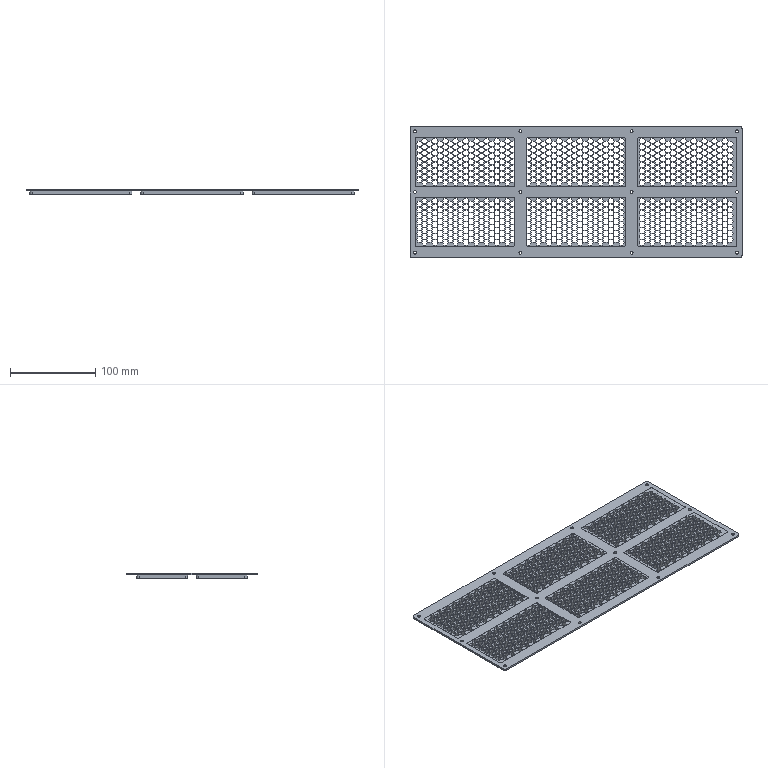NC program | NX | posted with a generic post
Lines 3670 to 4524 of 172913:
(CAVITY_MILL , TOOL : D3_ROUGH)
N7314 T12 M6
N7316 G54
N7318 G17 G0 G90 X-85.591 Y-50.877 S5500 M3
N7320 G43 Z20. H12
N7322 Z1.
N7324 G94 G1 X-85.511 Z0.998 F800.
N7326 X-84.68 Y-49.437 Z0.954
N7328 X-85.511 Y-47.997 Z0.911
N7330 X-87.174 Z0.867
N7332 X-88.006 Y-49.437 Z0.824
N7334 X-87.174 Y-50.877 Z0.78
N7336 X-85.511 Z0.737
N7338 X-84.68 Y-49.437 Z0.693
N7340 X-85.511 Y-47.997 Z0.65
N7342 X-87.174 Z0.606
N7344 X-88.006 Y-49.437 Z0.563
N7346 X-87.174 Y-50.877 Z0.519
N7348 X-85.511 Z0.475
N7350 X-84.68 Y-49.437 Z0.432
N7352 X-85.511 Y-47.997 Z0.388
N7354 X-87.174 Z0.345
N7356 X-88.006 Y-49.437 Z0.301
N7358 X-87.174 Y-50.877 Z0.258
N7360 X-85.511 Z0.214
N7362 X-84.68 Y-49.437 Z0.171
N7364 X-85.511 Y-47.997 Z0.127
N7366 X-87.174 Z0.084
N7368 X-88.006 Y-49.437 Z0.04
N7370 X-87.174 Y-50.877 Z-0.004
N7372 X-85.511 Z-0.047
N7374 X-84.68 Y-49.437 Z-0.091
N7376 X-85.511 Y-47.997 Z-0.134
N7378 X-87.174 Z-0.178
N7380 X-88.006 Y-49.437 Z-0.221
N7382 X-87.174 Y-50.877 Z-0.265
N7384 X-85.511 Z-0.308
N7386 X-84.68 Y-49.437 Z-0.352
N7388 X-85.511 Y-47.997 Z-0.395
N7390 X-87.174 Z-0.439
N7392 X-88.006 Y-49.437 Z-0.482
N7394 X-87.174 Y-50.877 Z-0.526
N7396 X-85.511 Z-0.57
N7398 X-84.68 Y-49.437 Z-0.613
N7400 X-85.511 Y-47.997 Z-0.657
N7402 X-87.174 Z-0.7
N7404 X-88.006 Y-49.437 Z-0.744
N7406 X-87.174 Y-50.877 Z-0.787
N7408 X-85.511 Z-0.831
N7410 X-84.68 Y-49.437 Z-0.874
N7412 X-85.511 Y-47.997 Z-0.918
N7414 X-87.174 Z-0.961
N7416 X-88.006 Y-49.437 Z-1.005
N7418 X-87.174 Y-50.877 Z-1.049
N7420 X-85.511 Z-1.092
N7422 X-84.68 Y-49.437 Z-1.136
N7424 X-85.511 Y-47.997 Z-1.179
N7426 X-87.174 Z-1.223
N7428 X-88.006 Y-49.437 Z-1.266
N7430 X-87.174 Y-50.877 Z-1.31
N7432 X-85.511 Z-1.353
N7434 X-84.68 Y-49.437 Z-1.397
N7436 X-85.511 Y-47.997 Z-1.44
N7438 X-87.174 Z-1.484
N7440 X-88.006 Y-49.437 Z-1.527
N7442 X-87.174 Y-50.877 Z-1.571
N7444 X-85.511 Z-1.615
N7446 X-84.68 Y-49.437 Z-1.658
N7448 X-85.511 Y-47.997 Z-1.702
N7450 X-87.174 Z-1.745
N7452 X-88.006 Y-49.437 Z-1.789
N7454 X-87.174 Y-50.877 Z-1.832
N7456 X-85.511 Z-1.876
N7458 X-84.68 Y-49.437 Z-1.919
N7460 X-85.511 Y-47.997 Z-1.963
N7462 X-87.174 Z-2.006
N7464 X-88.006 Y-49.437 Z-2.05
N7466 X-87.174 Y-50.877 Z-2.093
N7468 X-85.511 Z-2.137
N7470 X-84.68 Y-49.437 Z-2.181
N7472 X-85.511 Y-47.997 Z-2.224
N7474 X-87.174 Z-2.268
N7476 X-88.006 Y-49.437 Z-2.311
N7478 X-87.174 Y-50.877 Z-2.355
N7480 X-85.511 Z-2.398
N7482 X-84.68 Y-49.437 Z-2.442
N7484 X-85.511 Y-47.997 Z-2.485
N7486 X-87.174 Z-2.529
N7488 X-88.006 Y-49.437 Z-2.572
N7490 X-87.174 Y-50.877 Z-2.616
N7492 X-85.511 Z-2.66
N7494 X-84.68 Y-49.437 Z-2.703
N7496 X-85.511 Y-47.997 Z-2.747
N7498 X-87.174 Z-2.79
N7500 X-88.006 Y-49.437 Z-2.834
N7502 X-87.174 Y-50.877 Z-2.877
N7504 X-85.511 Z-2.921
N7506 X-84.68 Y-49.437 Z-2.964
N7508 X-85.511 Y-47.997 Z-3.008
N7510 X-87.174 Z-3.051
N7512 X-88.006 Y-49.437 Z-3.095
N7514 X-87.174 Y-50.877 Z-3.138
N7516 X-85.511 Z-3.182
N7518 X-84.68 Y-49.437 Z-3.226
N7520 X-85.511 Y-47.997 Z-3.269
N7522 X-87.174 Z-3.313
N7524 X-88.006 Y-49.437 Z-3.356
N7526 X-87.174 Y-50.877 Z-3.4
N7528 X-85.511 Z-3.443
N7530 X-84.68 Y-49.437 Z-3.487
N7532 X-85.511 Y-47.997 Z-3.53
N7534 X-87.174 Z-3.574
N7536 X-88.006 Y-49.437 Z-3.617
N7538 X-87.174 Y-50.877 Z-3.661
N7540 X-85.511 Z-3.705
N7542 X-84.68 Y-49.437 Z-3.748
N7544 X-85.511 Y-47.997 Z-3.792
N7546 X-87.174 Z-3.835
N7548 X-88.006 Y-49.437 Z-3.879
N7550 X-87.174 Y-50.877 Z-3.922
N7552 X-85.511 Z-3.966
N7554 X-84.68 Y-49.437 Z-4.009
N7556 X-85.511 Y-47.997 Z-4.053
N7558 X-87.174 Z-4.096
N7560 X-88.006 Y-49.437 Z-4.14
N7562 X-87.174 Y-50.877 Z-4.183
N7564 X-85.511 Z-4.227
N7566 X-84.68 Y-49.437 Z-4.271
N7568 X-85.511 Y-47.997 Z-4.314
N7570 X-87.174 Z-4.358
N7572 X-88.006 Y-49.437 Z-4.401
N7574 X-87.174 Y-50.877 Z-4.445
N7576 X-85.511 Z-4.488
N7578 X-84.68 Y-49.437 Z-4.532
N7580 X-85.511 Y-47.997 Z-4.575
N7582 X-87.174 Z-4.619
N7584 X-88.006 Y-49.437 Z-4.662
N7586 X-87.174 Y-50.877 Z-4.706
N7588 X-85.511 Z-4.75
N7590 X-84.68 Y-49.437 Z-4.793
N7592 X-85.511 Y-47.997 Z-4.837
N7594 X-87.174 Z-4.88
N7596 X-88.006 Y-49.437 Z-4.924
N7598 X-87.174 Y-50.877 Z-4.967
N7600 X-85.511 Z-5.011
N7602 X-84.68 Y-49.437 Z-5.054
N7604 X-85.511 Y-47.997 Z-5.098
N7606 X-87.174 Z-5.141
N7608 X-88.006 Y-49.437 Z-5.185
N7610 X-87.174 Y-50.877 Z-5.228
N7612 X-85.511 Z-5.272
N7614 X-84.68 Y-49.437 Z-5.316
N7616 X-85.511 Y-47.997 Z-5.359
N7618 X-87.174 Z-5.403
N7620 X-88.006 Y-49.437 Z-5.446
N7622 X-87.174 Y-50.877 Z-5.49
N7624 X-85.511 Z-5.533
N7626 X-84.68 Y-49.437 Z-5.577
N7628 X-85.511 Y-47.997 Z-5.62
N7630 X-87.174 Z-5.664
N7632 X-88.006 Y-49.437 Z-5.707
N7634 X-87.174 Y-50.877 Z-5.751
N7636 X-85.511 Z-5.794
N7638 X-84.68 Y-49.437 Z-5.838
N7640 X-85.511 Y-47.997 Z-5.882
N7642 X-87.174 Z-5.925
N7644 X-88.006 Y-49.437 Z-5.969
N7646 X-87.174 Y-50.877 Z-6.012
N7648 X-85.511 Z-6.056
N7650 X-84.68 Y-49.437 Z-6.099
N7652 X-85.511 Y-47.997 Z-6.143
N7654 X-87.174 Z-6.186
N7656 X-88.006 Y-49.437 Z-6.23
N7658 X-87.174 Y-50.877 Z-6.273
N7660 X-85.511 Z-6.317
N7662 X-84.68 Y-49.437 Z-6.361
N7664 X-85.511 Y-47.997 Z-6.404
N7666 X-87.174 Z-6.448
N7668 X-88.006 Y-49.437 Z-6.491
N7670 X-87.174 Y-50.877 Z-6.535
N7672 X-85.511 Z-6.578
N7674 X-85.096 Y-50.157 Z-6.6
N7676 X-84.68 Y-49.437
N7678 X-85.511 Y-47.997
N7680 X-87.174
N7682 X-88.006 Y-49.437
N7684 X-87.174 Y-50.877
N7686 X-85.511
N7688 X-85.096 Y-50.157
N7690 Z-5.6
N7692 G0 Z20.
N7694 X-87.214 Y-43.809
N7696 Z1.
N7698 G1 X-87.174 Y-43.877 Z0.998
N7700 X-85.511 Z0.954
N7702 X-84.68 Y-42.437 Z0.911
N7704 X-85.511 Y-40.997 Z0.867
N7706 X-87.174 Z0.824
N7708 X-88.006 Y-42.437 Z0.78
N7710 X-87.174 Y-43.877 Z0.737
N7712 X-85.511 Z0.693
N7714 X-84.68 Y-42.437 Z0.65
N7716 X-85.511 Y-40.997 Z0.606
N7718 X-87.174 Z0.563
N7720 X-88.006 Y-42.437 Z0.519
N7722 X-87.174 Y-43.877 Z0.475
N7724 X-85.511 Z0.432
N7726 X-84.68 Y-42.437 Z0.388
N7728 X-85.511 Y-40.997 Z0.345
N7730 X-87.174 Z0.301
N7732 X-88.006 Y-42.437 Z0.258
N7734 X-87.174 Y-43.877 Z0.214
N7736 X-85.511 Z0.171
N7738 X-84.68 Y-42.437 Z0.127
N7740 X-85.511 Y-40.997 Z0.084
N7742 X-87.174 Z0.04
N7744 X-88.006 Y-42.437 Z-0.004
N7746 X-87.174 Y-43.877 Z-0.047
N7748 X-85.511 Z-0.091
N7750 X-84.68 Y-42.437 Z-0.134
N7752 X-85.511 Y-40.997 Z-0.178
N7754 X-87.174 Z-0.221
N7756 X-88.006 Y-42.437 Z-0.265
N7758 X-87.174 Y-43.877 Z-0.308
N7760 X-85.511 Z-0.352
N7762 X-84.68 Y-42.437 Z-0.395
N7764 X-85.511 Y-40.997 Z-0.439
N7766 X-87.174 Z-0.482
N7768 X-88.006 Y-42.437 Z-0.526
N7770 X-87.174 Y-43.877 Z-0.57
N7772 X-85.511 Z-0.613
N7774 X-84.68 Y-42.437 Z-0.657
N7776 X-85.511 Y-40.997 Z-0.7
N7778 X-87.174 Z-0.744
N7780 X-88.006 Y-42.437 Z-0.787
N7782 X-87.174 Y-43.877 Z-0.831
N7784 X-85.511 Z-0.874
N7786 X-84.68 Y-42.437 Z-0.918
N7788 X-85.511 Y-40.997 Z-0.961
N7790 X-87.174 Z-1.005
N7792 X-88.006 Y-42.437 Z-1.049
N7794 X-87.174 Y-43.877 Z-1.092
N7796 X-85.511 Z-1.136
N7798 X-84.68 Y-42.437 Z-1.179
N7800 X-85.511 Y-40.997 Z-1.223
N7802 X-87.174 Z-1.266
N7804 X-88.006 Y-42.437 Z-1.31
N7806 X-87.174 Y-43.877 Z-1.353
N7808 X-85.511 Z-1.397
N7810 X-84.68 Y-42.437 Z-1.44
N7812 X-85.511 Y-40.997 Z-1.484
N7814 X-87.174 Z-1.527
N7816 X-88.006 Y-42.437 Z-1.571
N7818 X-87.174 Y-43.877 Z-1.615
N7820 X-85.511 Z-1.658
N7822 X-84.68 Y-42.437 Z-1.702
N7824 X-85.511 Y-40.997 Z-1.745
N7826 X-87.174 Z-1.789
N7828 X-88.006 Y-42.437 Z-1.832
N7830 X-87.174 Y-43.877 Z-1.876
N7832 X-85.511 Z-1.919
N7834 X-84.68 Y-42.437 Z-1.963
N7836 X-85.511 Y-40.997 Z-2.006
N7838 X-87.174 Z-2.05
N7840 X-88.006 Y-42.437 Z-2.093
N7842 X-87.174 Y-43.877 Z-2.137
N7844 X-85.511 Z-2.181
N7846 X-84.68 Y-42.437 Z-2.224
N7848 X-85.511 Y-40.997 Z-2.268
N7850 X-87.174 Z-2.311
N7852 X-88.006 Y-42.437 Z-2.355
N7854 X-87.174 Y-43.877 Z-2.398
N7856 X-85.511 Z-2.442
N7858 X-84.68 Y-42.437 Z-2.485
N7860 X-85.511 Y-40.997 Z-2.529
N7862 X-87.174 Z-2.572
N7864 X-88.006 Y-42.437 Z-2.616
N7866 X-87.174 Y-43.877 Z-2.66
N7868 X-85.511 Z-2.703
N7870 X-84.68 Y-42.437 Z-2.747
N7872 X-85.511 Y-40.997 Z-2.79
N7874 X-87.174 Z-2.834
N7876 X-88.006 Y-42.437 Z-2.877
N7878 X-87.174 Y-43.877 Z-2.921
N7880 X-85.511 Z-2.964
N7882 X-84.68 Y-42.437 Z-3.008
N7884 X-85.511 Y-40.997 Z-3.051
N7886 X-87.174 Z-3.095
N7888 X-88.006 Y-42.437 Z-3.138
N7890 X-87.174 Y-43.877 Z-3.182
N7892 X-85.511 Z-3.226
N7894 X-84.68 Y-42.437 Z-3.269
N7896 X-85.511 Y-40.997 Z-3.313
N7898 X-87.174 Z-3.356
N7900 X-88.006 Y-42.437 Z-3.4
N7902 X-87.174 Y-43.877 Z-3.443
N7904 X-85.511 Z-3.487
N7906 X-84.68 Y-42.437 Z-3.53
N7908 X-85.511 Y-40.997 Z-3.574
N7910 X-87.174 Z-3.617
N7912 X-88.006 Y-42.437 Z-3.661
N7914 X-87.174 Y-43.877 Z-3.705
N7916 X-85.511 Z-3.748
N7918 X-84.68 Y-42.437 Z-3.792
N7920 X-85.511 Y-40.997 Z-3.835
N7922 X-87.174 Z-3.879
N7924 X-88.006 Y-42.437 Z-3.922
N7926 X-87.174 Y-43.877 Z-3.966
N7928 X-85.511 Z-4.009
N7930 X-84.68 Y-42.437 Z-4.053
N7932 X-85.511 Y-40.997 Z-4.096
N7934 X-87.174 Z-4.14
N7936 X-88.006 Y-42.437 Z-4.183
N7938 X-87.174 Y-43.877 Z-4.227
N7940 X-85.511 Z-4.271
N7942 X-84.68 Y-42.437 Z-4.314
N7944 X-85.511 Y-40.997 Z-4.358
N7946 X-87.174 Z-4.401
N7948 X-88.006 Y-42.437 Z-4.445
N7950 X-87.174 Y-43.877 Z-4.488
N7952 X-85.511 Z-4.532
N7954 X-84.68 Y-42.437 Z-4.575
N7956 X-85.511 Y-40.997 Z-4.619
N7958 X-87.174 Z-4.662
N7960 X-88.006 Y-42.437 Z-4.706
N7962 X-87.174 Y-43.877 Z-4.75
N7964 X-85.511 Z-4.793
N7966 X-84.68 Y-42.437 Z-4.837
N7968 X-85.511 Y-40.997 Z-4.88
N7970 X-87.174 Z-4.924
N7972 X-88.006 Y-42.437 Z-4.967
N7974 X-87.174 Y-43.877 Z-5.011
N7976 X-85.511 Z-5.054
N7978 X-84.68 Y-42.437 Z-5.098
N7980 X-85.511 Y-40.997 Z-5.141
N7982 X-87.174 Z-5.185
N7984 X-88.006 Y-42.437 Z-5.228
N7986 X-87.174 Y-43.877 Z-5.272
N7988 X-85.511 Z-5.316
N7990 X-84.68 Y-42.437 Z-5.359
N7992 X-85.511 Y-40.997 Z-5.403
N7994 X-87.174 Z-5.446
N7996 X-88.006 Y-42.437 Z-5.49
N7998 X-87.174 Y-43.877 Z-5.533
N8000 X-85.511 Z-5.577
N8002 X-84.68 Y-42.437 Z-5.62
N8004 X-85.511 Y-40.997 Z-5.664
N8006 X-87.174 Z-5.707
N8008 X-88.006 Y-42.437 Z-5.751
N8010 X-87.174 Y-43.877 Z-5.794
N8012 X-85.511 Z-5.838
N8014 X-84.68 Y-42.437 Z-5.882
N8016 X-85.511 Y-40.997 Z-5.925
N8018 X-87.174 Z-5.969
N8020 X-88.006 Y-42.437 Z-6.012
N8022 X-87.174 Y-43.877 Z-6.056
N8024 X-85.511 Z-6.099
N8026 X-84.68 Y-42.437 Z-6.143
N8028 X-85.511 Y-40.997 Z-6.186
N8030 X-87.174 Z-6.23
N8032 X-88.006 Y-42.437 Z-6.273
N8034 X-87.174 Y-43.877 Z-6.317
N8036 X-85.511 Z-6.361
N8038 X-84.68 Y-42.437 Z-6.404
N8040 X-85.511 Y-40.997 Z-6.448
N8042 X-87.174 Z-6.491
N8044 X-88.006 Y-42.437 Z-6.535
N8046 X-87.174 Y-43.877 Z-6.578
N8048 X-86.343 Z-6.6
N8050 X-85.511
N8052 X-84.68 Y-42.437
N8054 X-85.511 Y-40.997
N8056 X-87.174
N8058 X-88.006 Y-42.437
N8060 X-87.174 Y-43.877
N8062 X-86.343
N8064 Z-5.6
N8066 G0 Z20.
N8068 X-91.653 Y-47.377
N8070 Z1.
N8072 G1 X-91.574 Z0.998
N8074 X-90.742 Y-45.937 Z0.954
N8076 X-91.574 Y-44.497 Z0.911
N8078 X-93.236 Z0.867
N8080 X-94.068 Y-45.937 Z0.824
N8082 X-93.236 Y-47.377 Z0.78
N8084 X-91.574 Z0.737
N8086 X-90.742 Y-45.937 Z0.693
N8088 X-91.574 Y-44.497 Z0.65
N8090 X-93.236 Z0.606
N8092 X-94.068 Y-45.937 Z0.563
N8094 X-93.236 Y-47.377 Z0.519
N8096 X-91.574 Z0.475
N8098 X-90.742 Y-45.937 Z0.432
N8100 X-91.574 Y-44.497 Z0.388
N8102 X-93.236 Z0.345
N8104 X-94.068 Y-45.937 Z0.301
N8106 X-93.236 Y-47.377 Z0.258
N8108 X-91.574 Z0.214
N8110 X-90.742 Y-45.937 Z0.171
N8112 X-91.574 Y-44.497 Z0.127
N8114 X-93.236 Z0.084
N8116 X-94.068 Y-45.937 Z0.04
N8118 X-93.236 Y-47.377 Z-0.004
N8120 X-91.574 Z-0.047
N8122 X-90.742 Y-45.937 Z-0.091
N8124 X-91.574 Y-44.497 Z-0.134
N8126 X-93.236 Z-0.178
N8128 X-94.068 Y-45.937 Z-0.221
N8130 X-93.236 Y-47.377 Z-0.265
N8132 X-91.574 Z-0.308
N8134 X-90.742 Y-45.937 Z-0.352
N8136 X-91.574 Y-44.497 Z-0.395
N8138 X-93.236 Z-0.439
N8140 X-94.068 Y-45.937 Z-0.482
N8142 X-93.236 Y-47.377 Z-0.526
N8144 X-91.574 Z-0.57
N8146 X-90.742 Y-45.937 Z-0.613
N8148 X-91.574 Y-44.497 Z-0.657
N8150 X-93.236 Z-0.7
N8152 X-94.068 Y-45.937 Z-0.744
N8154 X-93.236 Y-47.377 Z-0.787
N8156 X-91.574 Z-0.831
N8158 X-90.742 Y-45.937 Z-0.874
N8160 X-91.574 Y-44.497 Z-0.918
N8162 X-93.236 Z-0.961
N8164 X-94.068 Y-45.937 Z-1.005
N8166 X-93.236 Y-47.377 Z-1.049
N8168 X-91.574 Z-1.092
N8170 X-90.742 Y-45.937 Z-1.136
N8172 X-91.574 Y-44.497 Z-1.179
N8174 X-93.236 Z-1.223
N8176 X-94.068 Y-45.937 Z-1.266
N8178 X-93.236 Y-47.377 Z-1.31
N8180 X-91.574 Z-1.353
N8182 X-90.742 Y-45.937 Z-1.397
N8184 X-91.574 Y-44.497 Z-1.44
N8186 X-93.236 Z-1.484
N8188 X-94.068 Y-45.937 Z-1.527
N8190 X-93.236 Y-47.377 Z-1.571
N8192 X-91.574 Z-1.615
N8194 X-90.742 Y-45.937 Z-1.658
N8196 X-91.574 Y-44.497 Z-1.702
N8198 X-93.236 Z-1.745
N8200 X-94.068 Y-45.937 Z-1.789
N8202 X-93.236 Y-47.377 Z-1.832
N8204 X-91.574 Z-1.876
N8206 X-90.742 Y-45.937 Z-1.919
N8208 X-91.574 Y-44.497 Z-1.963
N8210 X-93.236 Z-2.006
N8212 X-94.068 Y-45.937 Z-2.05
N8214 X-93.236 Y-47.377 Z-2.093
N8216 X-91.574 Z-2.137
N8218 X-90.742 Y-45.937 Z-2.181
N8220 X-91.574 Y-44.497 Z-2.224
N8222 X-93.236 Z-2.268
N8224 X-94.068 Y-45.937 Z-2.311
N8226 X-93.236 Y-47.377 Z-2.355
N8228 X-91.574 Z-2.398
N8230 X-90.742 Y-45.937 Z-2.442
N8232 X-91.574 Y-44.497 Z-2.485
N8234 X-93.236 Z-2.529
N8236 X-94.068 Y-45.937 Z-2.572
N8238 X-93.236 Y-47.377 Z-2.616
N8240 X-91.574 Z-2.66
N8242 X-90.742 Y-45.937 Z-2.703
N8244 X-91.574 Y-44.497 Z-2.747
N8246 X-93.236 Z-2.79
N8248 X-94.068 Y-45.937 Z-2.834
N8250 X-93.236 Y-47.377 Z-2.877
N8252 X-91.574 Z-2.921
N8254 X-90.742 Y-45.937 Z-2.964
N8256 X-91.574 Y-44.497 Z-3.008
N8258 X-93.236 Z-3.051
N8260 X-94.068 Y-45.937 Z-3.095
N8262 X-93.236 Y-47.377 Z-3.138
N8264 X-91.574 Z-3.182
N8266 X-90.742 Y-45.937 Z-3.226
N8268 X-91.574 Y-44.497 Z-3.269
N8270 X-93.236 Z-3.313
N8272 X-94.068 Y-45.937 Z-3.356
N8274 X-93.236 Y-47.377 Z-3.4
N8276 X-91.574 Z-3.443
N8278 X-90.742 Y-45.937 Z-3.487
N8280 X-91.574 Y-44.497 Z-3.53
N8282 X-93.236 Z-3.574
N8284 X-94.068 Y-45.937 Z-3.617
N8286 X-93.236 Y-47.377 Z-3.661
N8288 X-91.574 Z-3.705
N8290 X-90.742 Y-45.937 Z-3.748
N8292 X-91.574 Y-44.497 Z-3.792
N8294 X-93.236 Z-3.835
N8296 X-94.068 Y-45.937 Z-3.879
N8298 X-93.236 Y-47.377 Z-3.922
N8300 X-91.574 Z-3.966
N8302 X-90.742 Y-45.937 Z-4.009
N8304 X-91.574 Y-44.497 Z-4.053
N8306 X-93.236 Z-4.096
N8308 X-94.068 Y-45.937 Z-4.14
N8310 X-93.236 Y-47.377 Z-4.183
N8312 X-91.574 Z-4.227
N8314 X-90.742 Y-45.937 Z-4.271
N8316 X-91.574 Y-44.497 Z-4.314
N8318 X-93.236 Z-4.358
N8320 X-94.068 Y-45.937 Z-4.401
N8322 X-93.236 Y-47.377 Z-4.445
N8324 X-91.574 Z-4.488
N8326 X-90.742 Y-45.937 Z-4.532
N8328 X-91.574 Y-44.497 Z-4.575
N8330 X-93.236 Z-4.619
N8332 X-94.068 Y-45.937 Z-4.662
N8334 X-93.236 Y-47.377 Z-4.706
N8336 X-91.574 Z-4.75
N8338 X-90.742 Y-45.937 Z-4.793
N8340 X-91.574 Y-44.497 Z-4.837
N8342 X-93.236 Z-4.88
N8344 X-94.068 Y-45.937 Z-4.924
N8346 X-93.236 Y-47.377 Z-4.967
N8348 X-91.574 Z-5.011
N8350 X-90.742 Y-45.937 Z-5.054
N8352 X-91.574 Y-44.497 Z-5.098
N8354 X-93.236 Z-5.141
N8356 X-94.068 Y-45.937 Z-5.185
N8358 X-93.236 Y-47.377 Z-5.228
N8360 X-91.574 Z-5.272
N8362 X-90.742 Y-45.937 Z-5.316
N8364 X-91.574 Y-44.497 Z-5.359
N8366 X-93.236 Z-5.403
N8368 X-94.068 Y-45.937 Z-5.446
N8370 X-93.236 Y-47.377 Z-5.49
N8372 X-91.574 Z-5.533
N8374 X-90.742 Y-45.937 Z-5.577
N8376 X-91.574 Y-44.497 Z-5.62
N8378 X-93.236 Z-5.664
N8380 X-94.068 Y-45.937 Z-5.707
N8382 X-93.236 Y-47.377 Z-5.751
N8384 X-91.574 Z-5.794
N8386 X-90.742 Y-45.937 Z-5.838
N8388 X-91.574 Y-44.497 Z-5.882
N8390 X-93.236 Z-5.925
N8392 X-94.068 Y-45.937 Z-5.969
N8394 X-93.236 Y-47.377 Z-6.012
N8396 X-91.574 Z-6.056
N8398 X-90.742 Y-45.937 Z-6.099
N8400 X-91.574 Y-44.497 Z-6.143
N8402 X-93.236 Z-6.186
N8404 X-94.068 Y-45.937 Z-6.23
N8406 X-93.236 Y-47.377 Z-6.273
N8408 X-91.574 Z-6.317
N8410 X-90.742 Y-45.937 Z-6.361
N8412 X-91.574 Y-44.497 Z-6.404
N8414 X-93.236 Z-6.448
N8416 X-94.068 Y-45.937 Z-6.491
N8418 X-93.236 Y-47.377 Z-6.535
N8420 X-91.574 Z-6.578
N8422 X-91.158 Y-46.657 Z-6.6
N8424 X-90.742 Y-45.937
N8426 X-91.574 Y-44.497
N8428 X-93.236
N8430 X-94.068 Y-45.937
N8432 X-93.236 Y-47.377
N8434 X-91.574
N8436 X-91.158 Y-46.657
N8438 Z-5.6
N8440 G0 Z20.
N8442 X-93.276 Y-54.309
N8444 Z1.
N8446 G1 X-93.236 Y-54.377 Z0.998
N8448 X-91.574 Z0.954
N8450 X-90.742 Y-52.937 Z0.911
N8452 X-91.574 Y-51.497 Z0.867
N8454 X-93.236 Z0.824
N8456 X-94.068 Y-52.937 Z0.78
N8458 X-93.236 Y-54.377 Z0.737
N8460 X-91.574 Z0.693
N8462 X-90.742 Y-52.937 Z0.65
N8464 X-91.574 Y-51.497 Z0.606
N8466 X-93.236 Z0.563
N8468 X-94.068 Y-52.937 Z0.519
N8470 X-93.236 Y-54.377 Z0.475
N8472 X-91.574 Z0.432
N8474 X-90.742 Y-52.937 Z0.388
N8476 X-91.574 Y-51.497 Z0.345
N8478 X-93.236 Z0.301
N8480 X-94.068 Y-52.937 Z0.258
N8482 X-93.236 Y-54.377 Z0.214
N8484 X-91.574 Z0.171
N8486 X-90.742 Y-52.937 Z0.127
N8488 X-91.574 Y-51.497 Z0.084
N8490 X-93.236 Z0.04
N8492 X-94.068 Y-52.937 Z-0.004
N8494 X-93.236 Y-54.377 Z-0.047
N8496 X-91.574 Z-0.091
N8498 X-90.742 Y-52.937 Z-0.134
N8500 X-91.574 Y-51.497 Z-0.178
N8502 X-93.236 Z-0.221
N8504 X-94.068 Y-52.937 Z-0.265
N8506 X-93.236 Y-54.377 Z-0.308
N8508 X-91.574 Z-0.352
N8510 X-90.742 Y-52.937 Z-0.395
N8512 X-91.574 Y-51.497 Z-0.439
N8514 X-93.236 Z-0.482
N8516 X-94.068 Y-52.937 Z-0.526
N8518 X-93.236 Y-54.377 Z-0.57
N8520 X-91.574 Z-0.613
N8522 X-90.742 Y-52.937 Z-0.657
N8524 X-91.574 Y-51.497 Z-0.7
N8526 X-93.236 Z-0.744
N8528 X-94.068 Y-52.937 Z-0.787
N8530 X-93.236 Y-54.377 Z-0.831
N8532 X-91.574 Z-0.874
N8534 X-90.742 Y-52.937 Z-0.918
N8536 X-91.574 Y-51.497 Z-0.961
N8538 X-93.236 Z-1.005
N8540 X-94.068 Y-52.937 Z-1.049
N8542 X-93.236 Y-54.377 Z-1.092
N8544 X-91.574 Z-1.136
N8546 X-90.742 Y-52.937 Z-1.179
N8548 X-91.574 Y-51.497 Z-1.223
N8550 X-93.236 Z-1.266
N8552 X-94.068 Y-52.937 Z-1.31
N8554 X-93.236 Y-54.377 Z-1.353
N8556 X-91.574 Z-1.397
N8558 X-90.742 Y-52.937 Z-1.44
N8560 X-91.574 Y-51.497 Z-1.484
N8562 X-93.236 Z-1.527
N8564 X-94.068 Y-52.937 Z-1.571
N8566 X-93.236 Y-54.377 Z-1.615
N8568 X-91.574 Z-1.658
N8570 X-90.742 Y-52.937 Z-1.702
N8572 X-91.574 Y-51.497 Z-1.745
N8574 X-93.236 Z-1.789
N8576 X-94.068 Y-52.937 Z-1.832
N8578 X-93.236 Y-54.377 Z-1.876
N8580 X-91.574 Z-1.919
N8582 X-90.742 Y-52.937 Z-1.963
N8584 X-91.574 Y-51.497 Z-2.006
N8586 X-93.236 Z-2.05
N8588 X-94.068 Y-52.937 Z-2.093
N8590 X-93.236 Y-54.377 Z-2.137
N8592 X-91.574 Z-2.181
N8594 X-90.742 Y-52.937 Z-2.224
N8596 X-91.574 Y-51.497 Z-2.268
N8598 X-93.236 Z-2.311
N8600 X-94.068 Y-52.937 Z-2.355
N8602 X-93.236 Y-54.377 Z-2.398
N8604 X-91.574 Z-2.442
N8606 X-90.742 Y-52.937 Z-2.485
N8608 X-91.574 Y-51.497 Z-2.529
N8610 X-93.236 Z-2.572
N8612 X-94.068 Y-52.937 Z-2.616
N8614 X-93.236 Y-54.377 Z-2.66
N8616 X-91.574 Z-2.703
N8618 X-90.742 Y-52.937 Z-2.747
N8620 X-91.574 Y-51.497 Z-2.79
N8622 X-93.236 Z-2.834
N8624 X-94.068 Y-52.937 Z-2.877
N8626 X-93.236 Y-54.377 Z-2.921
N8628 X-91.574 Z-2.964
N8630 X-90.742 Y-52.937 Z-3.008
N8632 X-91.574 Y-51.497 Z-3.051
N8634 X-93.236 Z-3.095
N8636 X-94.068 Y-52.937 Z-3.138
N8638 X-93.236 Y-54.377 Z-3.182
N8640 X-91.574 Z-3.226
N8642 X-90.742 Y-52.937 Z-3.269
N8644 X-91.574 Y-51.497 Z-3.313
N8646 X-93.236 Z-3.356
N8648 X-94.068 Y-52.937 Z-3.4
N8650 X-93.236 Y-54.377 Z-3.443
N8652 X-91.574 Z-3.487
N8654 X-90.742 Y-52.937 Z-3.53
N8656 X-91.574 Y-51.497 Z-3.574
N8658 X-93.236 Z-3.617
N8660 X-94.068 Y-52.937 Z-3.661
N8662 X-93.236 Y-54.377 Z-3.705
N8664 X-91.574 Z-3.748
N8666 X-90.742 Y-52.937 Z-3.792
N8668 X-91.574 Y-51.497 Z-3.835
N8670 X-93.236 Z-3.879
N8672 X-94.068 Y-52.937 Z-3.922
N8674 X-93.236 Y-54.377 Z-3.966
N8676 X-91.574 Z-4.009
N8678 X-90.742 Y-52.937 Z-4.053
N8680 X-91.574 Y-51.497 Z-4.096
N8682 X-93.236 Z-4.14
N8684 X-94.068 Y-52.937 Z-4.183
N8686 X-93.236 Y-54.377 Z-4.227
N8688 X-91.574 Z-4.271
N8690 X-90.742 Y-52.937 Z-4.314
N8692 X-91.574 Y-51.497 Z-4.358
N8694 X-93.236 Z-4.401
N8696 X-94.068 Y-52.937 Z-4.445
N8698 X-93.236 Y-54.377 Z-4.488
N8700 X-91.574 Z-4.532
N8702 X-90.742 Y-52.937 Z-4.575
N8704 X-91.574 Y-51.497 Z-4.619
N8706 X-93.236 Z-4.662
N8708 X-94.068 Y-52.937 Z-4.706
N8710 X-93.236 Y-54.377 Z-4.75
N8712 X-91.574 Z-4.793
N8714 X-90.742 Y-52.937 Z-4.837
N8716 X-91.574 Y-51.497 Z-4.88
N8718 X-93.236 Z-4.924
N8720 X-94.068 Y-52.937 Z-4.967
N8722 X-93.236 Y-54.377 Z-5.011
N8724 X-91.574 Z-5.054
N8726 X-90.742 Y-52.937 Z-5.098
N8728 X-91.574 Y-51.497 Z-5.141
N8730 X-93.236 Z-5.185
N8732 X-94.068 Y-52.937 Z-5.228
N8734 X-93.236 Y-54.377 Z-5.272
N8736 X-91.574 Z-5.316
N8738 X-90.742 Y-52.937 Z-5.359
N8740 X-91.574 Y-51.497 Z-5.403
N8742 X-93.236 Z-5.446
N8744 X-94.068 Y-52.937 Z-5.49
N8746 X-93.236 Y-54.377 Z-5.533
N8748 X-91.574 Z-5.577
N8750 X-90.742 Y-52.937 Z-5.62
N8752 X-91.574 Y-51.497 Z-5.664
N8754 X-93.236 Z-5.707
N8756 X-94.068 Y-52.937 Z-5.751
N8758 X-93.236 Y-54.377 Z-5.794
N8760 X-91.574 Z-5.838
N8762 X-90.742 Y-52.937 Z-5.882
N8764 X-91.574 Y-51.497 Z-5.925
N8766 X-93.236 Z-5.969
N8768 X-94.068 Y-52.937 Z-6.012
N8770 X-93.236 Y-54.377 Z-6.056
N8772 X-91.574 Z-6.099
N8774 X-90.742 Y-52.937 Z-6.143
N8776 X-91.574 Y-51.497 Z-6.186
N8778 X-93.236 Z-6.23
N8780 X-94.068 Y-52.937 Z-6.273
N8782 X-93.236 Y-54.377 Z-6.317
N8784 X-91.574 Z-6.361
N8786 X-90.742 Y-52.937 Z-6.404
N8788 X-91.574 Y-51.497 Z-6.448
N8790 X-93.236 Z-6.491
N8792 X-94.068 Y-52.937 Z-6.535
N8794 X-93.236 Y-54.377 Z-6.578
N8796 X-92.405 Z-6.6
N8798 X-91.574
N8800 X-90.742 Y-52.937
N8802 X-91.574 Y-51.497
N8804 X-93.236
N8806 X-94.068 Y-52.937
N8808 X-93.236 Y-54.377
N8810 X-92.405
N8812 Z-5.6
N8814 G0 Z20.
N8816 X-93.276 Y-61.309
N8818 Z1.
N8820 G1 X-93.236 Y-61.377 Z0.998
N8822 X-91.574 Z0.954
N8824 X-90.742 Y-59.937 Z0.911
N8826 X-91.574 Y-58.497 Z0.867
N8828 X-93.236 Z0.824
N8830 X-94.068 Y-59.937 Z0.78
N8832 X-93.236 Y-61.377 Z0.737
N8834 X-91.574 Z0.693
N8836 X-90.742 Y-59.937 Z0.65
N8838 X-91.574 Y-58.497 Z0.606
N8840 X-93.236 Z0.563
N8842 X-94.068 Y-59.937 Z0.519
N8844 X-93.236 Y-61.377 Z0.475
N8846 X-91.574 Z0.432
N8848 X-90.742 Y-59.937 Z0.388
N8850 X-91.574 Y-58.497 Z0.345
N8852 X-93.236 Z0.301
N8854 X-94.068 Y-59.937 Z0.258
N8856 X-93.236 Y-61.377 Z0.214
N8858 X-91.574 Z0.171
N8860 X-90.742 Y-59.937 Z0.127
N8862 X-91.574 Y-58.497 Z0.084
N8864 X-93.236 Z0.04
N8866 X-94.068 Y-59.937 Z-0.004
N8868 X-93.236 Y-61.377 Z-0.047
N8870 X-91.574 Z-0.091
N8872 X-90.742 Y-59.937 Z-0.134
N8874 X-91.574 Y-58.497 Z-0.178
N8876 X-93.236 Z-0.221
N8878 X-94.068 Y-59.937 Z-0.265
N8880 X-93.236 Y-61.377 Z-0.308
N8882 X-91.574 Z-0.352
N8884 X-90.742 Y-59.937 Z-0.395
N8886 X-91.574 Y-58.497 Z-0.439
N8888 X-93.236 Z-0.482
N8890 X-94.068 Y-59.937 Z-0.526
N8892 X-93.236 Y-61.377 Z-0.57
N8894 X-91.574 Z-0.613
N8896 X-90.742 Y-59.937 Z-0.657
N8898 X-91.574 Y-58.497 Z-0.7
N8900 X-93.236 Z-0.744
N8902 X-94.068 Y-59.937 Z-0.787
N8904 X-93.236 Y-61.377 Z-0.831
N8906 X-91.574 Z-0.874
N8908 X-90.742 Y-59.937 Z-0.918
N8910 X-91.574 Y-58.497 Z-0.961
N8912 X-93.236 Z-1.005
N8914 X-94.068 Y-59.937 Z-1.049
N8916 X-93.236 Y-61.377 Z-1.092
N8918 X-91.574 Z-1.136
N8920 X-90.742 Y-59.937 Z-1.179
N8922 X-91.574 Y-58.497 Z-1.223
N8924 X-93.236 Z-1.266
N8926 X-94.068 Y-59.937 Z-1.31
N8928 X-93.236 Y-61.377 Z-1.353
N8930 X-91.574 Z-1.397
N8932 X-90.742 Y-59.937 Z-1.44
N8934 X-91.574 Y-58.497 Z-1.484
N8936 X-93.236 Z-1.527
N8938 X-94.068 Y-59.937 Z-1.571
N8940 X-93.236 Y-61.377 Z-1.615
N8942 X-91.574 Z-1.658
N8944 X-90.742 Y-59.937 Z-1.702
N8946 X-91.574 Y-58.497 Z-1.745
N8948 X-93.236 Z-1.789
N8950 X-94.068 Y-59.937 Z-1.832
N8952 X-93.236 Y-61.377 Z-1.876
N8954 X-91.574 Z-1.919
N8956 X-90.742 Y-59.937 Z-1.963
N8958 X-91.574 Y-58.497 Z-2.006
N8960 X-93.236 Z-2.05
N8962 X-94.068 Y-59.937 Z-2.093
N8964 X-93.236 Y-61.377 Z-2.137
N8966 X-91.574 Z-2.181
N8968 X-90.742 Y-59.937 Z-2.224
N8970 X-91.574 Y-58.497 Z-2.268
N8972 X-93.236 Z-2.311
N8974 X-94.068 Y-59.937 Z-2.355
N8976 X-93.236 Y-61.377 Z-2.398
N8978 X-91.574 Z-2.442
N8980 X-90.742 Y-59.937 Z-2.485
N8982 X-91.574 Y-58.497 Z-2.529
N8984 X-93.236 Z-2.572
N8986 X-94.068 Y-59.937 Z-2.616
N8988 X-93.236 Y-61.377 Z-2.66
N8990 X-91.574 Z-2.703
N8992 X-90.742 Y-59.937 Z-2.747
N8994 X-91.574 Y-58.497 Z-2.79
N8996 X-93.236 Z-2.834
N8998 X-94.068 Y-59.937 Z-2.877
N9000 X-93.236 Y-61.377 Z-2.921
N9002 X-91.574 Z-2.964
N9004 X-90.742 Y-59.937 Z-3.008
N9006 X-91.574 Y-58.497 Z-3.051
N9008 X-93.236 Z-3.095
N9010 X-94.068 Y-59.937 Z-3.138
N9012 X-93.236 Y-61.377 Z-3.182
N9014 X-91.574 Z-3.226
N9016 X-90.742 Y-59.937 Z-3.269